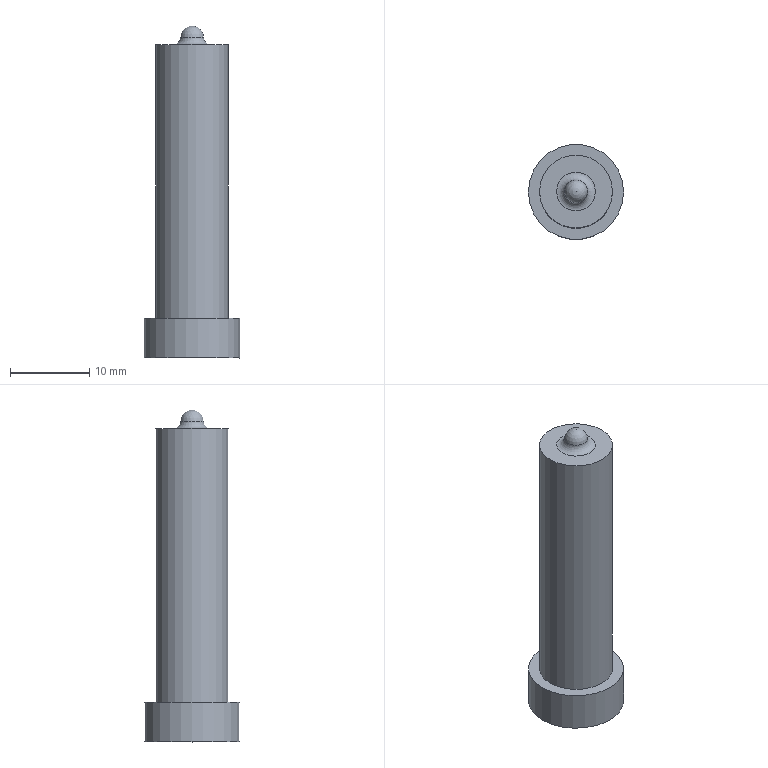Part | NX | features solid 2 | 1 solid | 7 faces | box 12 x 12 x 41.85 mm | volume 2873 mm3 | plane 3 | cylinder 2 | sphere 1 | torus 1 | commonest cylinder face diameters 9.2 x1 12 x1
STEP:
#1=CARTESIAN_POINT('',(3263.866,-906.707,863.216));
#2=VERTEX_POINT('',#1);
#3=CARTESIAN_POINT('',(3259.266,-906.707,863.216));
#4=DIRECTION('',(0.,0.,1.));
#5=DIRECTION('',(1.,0.,0.));
#6=AXIS2_PLACEMENT_3D('',#3,#4,#5);
#7=CIRCLE('',#6,4.6);
#8=EDGE_CURVE('',#2,#2,#7,.F.);
#9=ORIENTED_EDGE('',*,*,#8,.T.);
#10=EDGE_LOOP('',(#9));
#11=FACE_BOUND('',#10,.T.);
#12=CARTESIAN_POINT('',(3254.666,-906.707,828.716));
#13=VERTEX_POINT('',#12);
#14=CARTESIAN_POINT('',(3259.266,-906.707,828.716));
#15=DIRECTION('',(0.,0.,-1.));
#16=DIRECTION('',(-1.,0.,0.));
#17=AXIS2_PLACEMENT_3D('',#14,#15,#16);
#18=CIRCLE('',#17,4.6);
#19=EDGE_CURVE('',#13,#13,#18,.F.);
#20=ORIENTED_EDGE('',*,*,#19,.T.);
#21=EDGE_LOOP('',(#20));
#22=FACE_BOUND('',#21,.T.);
#23=CARTESIAN_POINT('',(3259.266,-906.707,863.216));
#24=DIRECTION('',(0.,0.,-1.));
#25=DIRECTION('',(1.,0.,0.));
#26=AXIS2_PLACEMENT_3D('',#23,#24,#25);
#27=CYLINDRICAL_SURFACE('',#26,4.6);
#28=ADVANCED_FACE('',(#11,#22),#27,.T.);
#29=CARTESIAN_POINT('',(3261.714,-906.707,863.216));
#30=VERTEX_POINT('',#29);
#31=CARTESIAN_POINT('',(3259.266,-906.707,863.216));
#32=DIRECTION('',(0.,0.,1.));
#33=DIRECTION('',(1.,0.,0.));
#34=AXIS2_PLACEMENT_3D('',#31,#32,#33);
#35=CIRCLE('',#34,2.448);
#36=EDGE_CURVE('',#30,#30,#35,.F.);
#37=ORIENTED_EDGE('',*,*,#36,.T.);
#38=EDGE_LOOP('',(#37));
#39=FACE_BOUND('',#38,.T.);
#40=ORIENTED_EDGE('',*,*,#8,.F.);
#41=EDGE_LOOP('',(#40));
#42=FACE_BOUND('',#41,.T.);
#43=CARTESIAN_POINT('',(3259.266,-906.707,863.216));
#44=DIRECTION('',(0.,0.,1.));
#45=DIRECTION('',(1.,0.,0.));
#46=AXIS2_PLACEMENT_3D('',#43,#44,#45);
#47=PLANE('',#46);
#48=ADVANCED_FACE('',(#39,#42),#47,.T.);
#49=CARTESIAN_POINT('',(3253.266,-906.707,823.716));
#50=VERTEX_POINT('',#49);
#51=CARTESIAN_POINT('',(3259.266,-906.707,823.716));
#52=DIRECTION('',(0.,0.,-1.));
#53=DIRECTION('',(-1.,0.,0.));
#54=AXIS2_PLACEMENT_3D('',#51,#52,#53);
#55=CIRCLE('',#54,6.);
#56=EDGE_CURVE('',#50,#50,#55,.T.);
#57=ORIENTED_EDGE('',*,*,#56,.T.);
#58=EDGE_LOOP('',(#57));
#59=FACE_BOUND('',#58,.T.);
#60=CARTESIAN_POINT('',(3035.264,-907.381,823.716));
#61=DIRECTION('',(0.,0.,-1.));
#62=DIRECTION('',(-1.,0.,0.));
#63=AXIS2_PLACEMENT_3D('',#60,#61,#62);
#64=PLANE('',#63);
#65=ADVANCED_FACE('',(#59),#64,.T.);
#66=CARTESIAN_POINT('',(3253.266,-906.707,828.716));
#67=VERTEX_POINT('',#66);
#68=CARTESIAN_POINT('',(3259.266,-906.707,828.716));
#69=DIRECTION('',(0.,0.,-1.));
#70=DIRECTION('',(-1.,0.,0.));
#71=AXIS2_PLACEMENT_3D('',#68,#69,#70);
#72=CIRCLE('',#71,6.);
#73=EDGE_CURVE('',#67,#67,#72,.T.);
#74=ORIENTED_EDGE('',*,*,#73,.T.);
#75=EDGE_LOOP('',(#74));
#76=FACE_BOUND('',#75,.T.);
#77=ORIENTED_EDGE('',*,*,#56,.F.);
#78=EDGE_LOOP('',(#77));
#79=FACE_BOUND('',#78,.T.);
#80=CARTESIAN_POINT('',(3259.266,-906.707,863.216));
#81=DIRECTION('',(0.,0.,-1.));
#82=DIRECTION('',(1.,0.,0.));
#83=AXIS2_PLACEMENT_3D('',#80,#81,#82);
#84=CYLINDRICAL_SURFACE('',#83,6.);
#85=ADVANCED_FACE('',(#76,#79),#84,.T.);
#86=ORIENTED_EDGE('',*,*,#19,.F.);
#87=EDGE_LOOP('',(#86));
#88=FACE_BOUND('',#87,.T.);
#89=ORIENTED_EDGE('',*,*,#73,.F.);
#90=EDGE_LOOP('',(#89));
#91=FACE_BOUND('',#90,.T.);
#92=CARTESIAN_POINT('',(3259.266,-906.707,828.716));
#93=DIRECTION('',(0.,0.,-1.));
#94=DIRECTION('',(-1.,0.,0.));
#95=AXIS2_PLACEMENT_3D('',#92,#93,#94);
#96=PLANE('',#95);
#97=ADVANCED_FACE('',(#88,#91),#96,.F.);
#98=CARTESIAN_POINT('',(3257.817,-906.707,864.175));
#99=VERTEX_POINT('',#98);
#100=CARTESIAN_POINT('',(3259.266,-906.707,864.175));
#101=DIRECTION('',(0.,0.,-1.));
#102=DIRECTION('',(-1.,0.,0.));
#103=AXIS2_PLACEMENT_3D('',#100,#101,#102);
#104=CIRCLE('',#103,1.449);
#105=EDGE_CURVE('',#99,#99,#104,.F.);
#106=ORIENTED_EDGE('',*,*,#105,.T.);
#107=EDGE_LOOP('',(#106));
#108=FACE_BOUND('',#107,.T.);
#109=CARTESIAN_POINT('',(3259.266,-906.707,864.116));
#110=DIRECTION('',(0.,0.,1.));
#111=DIRECTION('',(1.,0.,0.));
#112=AXIS2_PLACEMENT_3D('',#109,#110,#111);
#113=SPHERICAL_SURFACE('',#112,1.45);
#114=ADVANCED_FACE('',(#108),#113,.T.);
#115=ORIENTED_EDGE('',*,*,#36,.F.);
#116=EDGE_LOOP('',(#115));
#117=FACE_BOUND('',#116,.T.);
#118=ORIENTED_EDGE('',*,*,#105,.F.);
#119=EDGE_LOOP('',(#118));
#120=FACE_BOUND('',#119,.T.);
#121=CARTESIAN_POINT('',(3259.266,-906.707,864.216));
#122=DIRECTION('',(0.,0.,1.));
#123=DIRECTION('',(1.,0.,0.));
#124=AXIS2_PLACEMENT_3D('',#121,#122,#123);
#125=TOROIDAL_SURFACE('',#124,2.448,1.);
#126=ADVANCED_FACE('',(#117,#120),#125,.F.);
#127=CLOSED_SHELL('',(#28,#48,#65,#85,#97,#114,#126));
#128=MANIFOLD_SOLID_BREP('',#127);
#129=(LENGTH_UNIT()NAMED_UNIT(*)SI_UNIT(.MILLI.,.METRE.));
#130=UNCERTAINTY_MEASURE_WITH_UNIT(LENGTH_MEASURE(0.00001),#129,'','');
#131=(NAMED_UNIT(*)PLANE_ANGLE_UNIT()SI_UNIT($,.RADIAN.));
#132=(NAMED_UNIT(*)SI_UNIT($,.STERADIAN.)SOLID_ANGLE_UNIT());
#133=(GEOMETRIC_REPRESENTATION_CONTEXT(3)GLOBAL_UNCERTAINTY_ASSIGNED_CONTEXT((#130))GLOBAL_UNIT_ASSIGNED_CONTEXT((#129,#131,#132))REPRESENTATION_CONTEXT('',''));
#134=ADVANCED_BREP_SHAPE_REPRESENTATION('',(#128),#133);